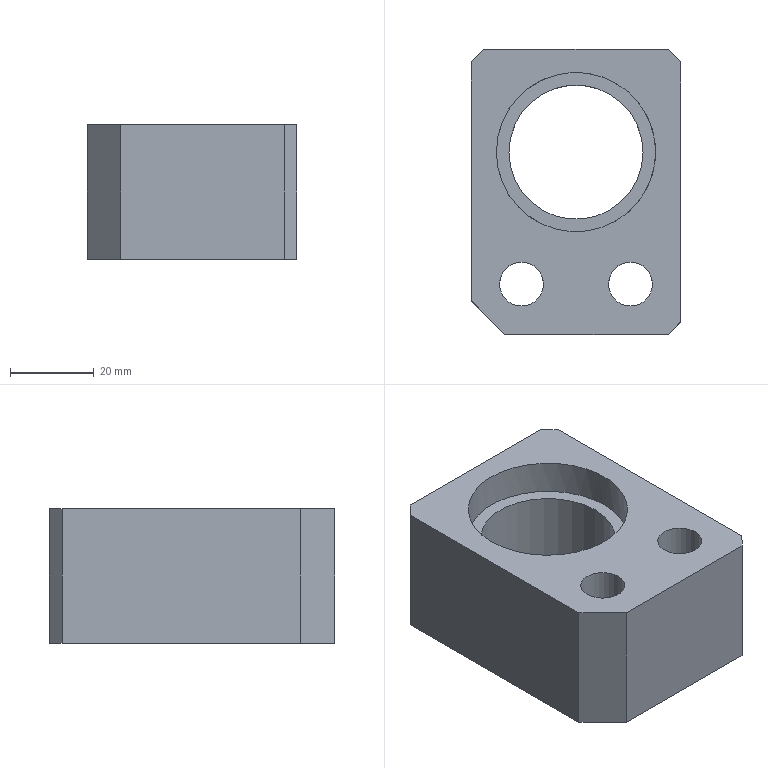Part | STEP file | lll_id3542_x_t | 1 solid | 19 faces | box 50 x 68 x 32 mm | volume 68588 mm3 | plane 13 | cylinder 6 | commonest cylinder face diameters 10.5 x2 17 x2 32 x1 38 x1
STEP:
#1=CARTESIAN_POINT('',(3217.117,-235.788,77.5));
#2=VERTEX_POINT('',#1);
#3=CARTESIAN_POINT('',(3222.367,-235.788,77.5));
#4=DIRECTION('',(0.,0.,1.));
#5=DIRECTION('',(-1.,0.,0.));
#6=AXIS2_PLACEMENT_3D('',#3,#4,#5);
#7=CIRCLE('',#6,5.25);
#8=EDGE_CURVE('',#2,#2,#7,.T.);
#9=ORIENTED_EDGE('',*,*,#8,.T.);
#10=EDGE_LOOP('',(#9));
#11=FACE_BOUND('',#10,.T.);
#12=CARTESIAN_POINT('',(3213.867,-235.788,77.5));
#13=VERTEX_POINT('',#12);
#14=CARTESIAN_POINT('',(3222.367,-235.788,77.5));
#15=DIRECTION('',(0.,0.,1.));
#16=DIRECTION('',(-1.,0.,0.));
#17=AXIS2_PLACEMENT_3D('',#14,#15,#16);
#18=CIRCLE('',#17,8.5);
#19=EDGE_CURVE('',#13,#13,#18,.T.);
#20=ORIENTED_EDGE('',*,*,#19,.F.);
#21=EDGE_LOOP('',(#20));
#22=FACE_BOUND('',#21,.T.);
#23=CARTESIAN_POINT('',(3222.367,-235.788,77.5));
#24=DIRECTION('',(0.,0.,1.));
#25=DIRECTION('',(1.,0.,0.));
#26=AXIS2_PLACEMENT_3D('',#23,#24,#25);
#27=PLANE('',#26);
#28=ADVANCED_FACE('',(#11,#22),#27,.F.);
#29=CARTESIAN_POINT('',(3254.367,-204.288,84.3));
#30=VERTEX_POINT('',#29);
#31=CARTESIAN_POINT('',(3235.367,-204.288,84.3));
#32=DIRECTION('',(0.,0.,1.));
#33=DIRECTION('',(1.,0.,0.));
#34=AXIS2_PLACEMENT_3D('',#31,#32,#33);
#35=CIRCLE('',#34,19.);
#36=EDGE_CURVE('',#30,#30,#35,.T.);
#37=ORIENTED_EDGE('',*,*,#36,.T.);
#38=EDGE_LOOP('',(#37));
#39=FACE_BOUND('',#38,.T.);
#40=CARTESIAN_POINT('',(3251.367,-204.288,84.3));
#41=VERTEX_POINT('',#40);
#42=CARTESIAN_POINT('',(3235.367,-204.288,84.3));
#43=DIRECTION('',(0.,0.,1.));
#44=DIRECTION('',(1.,0.,0.));
#45=AXIS2_PLACEMENT_3D('',#42,#43,#44);
#46=CIRCLE('',#45,16.);
#47=EDGE_CURVE('',#41,#41,#46,.T.);
#48=ORIENTED_EDGE('',*,*,#47,.F.);
#49=EDGE_LOOP('',(#48));
#50=FACE_BOUND('',#49,.T.);
#51=CARTESIAN_POINT('',(3235.367,-213.038,84.3));
#52=DIRECTION('',(0.,0.,-1.));
#53=DIRECTION('',(0.,-1.,0.));
#54=AXIS2_PLACEMENT_3D('',#51,#52,#53);
#55=PLANE('',#54);
#56=ADVANCED_FACE('',(#39,#50),#55,.F.);
#57=ORIENTED_EDGE('',*,*,#19,.T.);
#58=EDGE_LOOP('',(#57));
#59=FACE_BOUND('',#58,.T.);
#60=CARTESIAN_POINT('',(3213.867,-235.788,60.5));
#61=VERTEX_POINT('',#60);
#62=CARTESIAN_POINT('',(3222.367,-235.788,60.5));
#63=DIRECTION('',(0.,0.,-1.));
#64=DIRECTION('',(-1.,0.,0.));
#65=AXIS2_PLACEMENT_3D('',#62,#63,#64);
#66=CIRCLE('',#65,8.5);
#67=EDGE_CURVE('',#61,#61,#66,.T.);
#68=ORIENTED_EDGE('',*,*,#67,.T.);
#69=EDGE_LOOP('',(#68));
#70=FACE_BOUND('',#69,.T.);
#71=CARTESIAN_POINT('',(3222.367,-235.788,60.5));
#72=DIRECTION('',(0.,0.,1.));
#73=DIRECTION('',(1.,0.,0.));
#74=AXIS2_PLACEMENT_3D('',#71,#72,#73);
#75=CYLINDRICAL_SURFACE('',#74,8.5);
#76=ADVANCED_FACE('',(#59,#70),#75,.F.);
#77=CARTESIAN_POINT('',(3210.367,-182.788,60.5));
#78=VERTEX_POINT('',#77);
#79=CARTESIAN_POINT('',(3213.367,-179.788,60.5));
#80=VERTEX_POINT('',#79);
#81=CARTESIAN_POINT('',(3229.549,-163.605,60.5));
#82=DIRECTION('',(0.7071,0.7071,0.));
#83=VECTOR('',#82,1.);
#84=LINE('',#81,#83);
#85=EDGE_CURVE('',#78,#80,#84,.T.);
#86=ORIENTED_EDGE('',*,*,#85,.F.);
#87=CARTESIAN_POINT('',(3210.367,-182.788,92.5));
#88=VERTEX_POINT('',#87);
#89=CARTESIAN_POINT('',(3210.367,-182.788,-8.5));
#90=DIRECTION('',(0.,0.,-1.));
#91=VECTOR('',#90,1.);
#92=LINE('',#89,#91);
#93=EDGE_CURVE('',#88,#78,#92,.T.);
#94=ORIENTED_EDGE('',*,*,#93,.F.);
#95=CARTESIAN_POINT('',(3213.367,-179.788,92.5));
#96=VERTEX_POINT('',#95);
#97=CARTESIAN_POINT('',(3229.549,-163.605,92.5));
#98=DIRECTION('',(-0.7071,-0.7071,0.));
#99=VECTOR('',#98,1.);
#100=LINE('',#97,#99);
#101=EDGE_CURVE('',#96,#88,#100,.T.);
#102=ORIENTED_EDGE('',*,*,#101,.F.);
#103=CARTESIAN_POINT('',(3213.367,-179.788,-8.5));
#104=DIRECTION('',(0.,0.,1.));
#105=VECTOR('',#104,1.);
#106=LINE('',#103,#105);
#107=EDGE_CURVE('',#80,#96,#106,.T.);
#108=ORIENTED_EDGE('',*,*,#107,.F.);
#109=EDGE_LOOP('',(#86,#94,#102,#108));
#110=FACE_OUTER_BOUND('',#109,.T.);
#111=CARTESIAN_POINT('',(3213.367,-179.788,-8.5));
#112=DIRECTION('',(0.7071,-0.7071,0.));
#113=DIRECTION('',(0.,0.,1.));
#114=AXIS2_PLACEMENT_3D('',#111,#112,#113);
#115=PLANE('',#114);
#116=ADVANCED_FACE('',(#110),#115,.F.);
#117=CARTESIAN_POINT('',(3257.367,-179.788,60.5));
#118=VERTEX_POINT('',#117);
#119=CARTESIAN_POINT('',(3298.557,-179.788,60.5));
#120=DIRECTION('',(1.,0.,0.));
#121=VECTOR('',#120,1.);
#122=LINE('',#119,#121);
#123=EDGE_CURVE('',#80,#118,#122,.T.);
#124=ORIENTED_EDGE('',*,*,#123,.F.);
#125=ORIENTED_EDGE('',*,*,#107,.T.);
#126=CARTESIAN_POINT('',(3257.367,-179.788,92.5));
#127=VERTEX_POINT('',#126);
#128=CARTESIAN_POINT('',(3235.367,-179.788,92.5));
#129=DIRECTION('',(-1.,0.,0.));
#130=VECTOR('',#129,1.);
#131=LINE('',#128,#130);
#132=EDGE_CURVE('',#127,#96,#131,.T.);
#133=ORIENTED_EDGE('',*,*,#132,.F.);
#134=CARTESIAN_POINT('',(3257.367,-179.788,-8.5));
#135=DIRECTION('',(0.,0.,1.));
#136=VECTOR('',#135,1.);
#137=LINE('',#134,#136);
#138=EDGE_CURVE('',#118,#127,#137,.T.);
#139=ORIENTED_EDGE('',*,*,#138,.F.);
#140=EDGE_LOOP('',(#124,#125,#133,#139));
#141=FACE_OUTER_BOUND('',#140,.T.);
#142=CARTESIAN_POINT('',(3235.367,-179.788,-8.5));
#143=DIRECTION('',(0.,1.,0.));
#144=DIRECTION('',(0.,0.,-1.));
#145=AXIS2_PLACEMENT_3D('',#142,#143,#144);
#146=PLANE('',#145);
#147=ADVANCED_FACE('',(#141),#146,.T.);
#148=CARTESIAN_POINT('',(3260.367,-182.788,92.5));
#149=VERTEX_POINT('',#148);
#150=CARTESIAN_POINT('',(3260.367,-182.788,92.5));
#151=DIRECTION('',(0.7071,-0.7071,0.));
#152=VECTOR('',#151,1.);
#153=LINE('',#150,#152);
#154=EDGE_CURVE('',#127,#149,#153,.T.);
#155=ORIENTED_EDGE('',*,*,#154,.T.);
#156=CARTESIAN_POINT('',(3260.367,-182.788,60.5));
#157=VERTEX_POINT('',#156);
#158=CARTESIAN_POINT('',(3260.367,-182.788,-8.5));
#159=DIRECTION('',(0.,0.,-1.));
#160=VECTOR('',#159,1.);
#161=LINE('',#158,#160);
#162=EDGE_CURVE('',#149,#157,#161,.T.);
#163=ORIENTED_EDGE('',*,*,#162,.T.);
#164=CARTESIAN_POINT('',(3255.417,-177.838,60.5));
#165=DIRECTION('',(-0.7071,0.7071,0.));
#166=VECTOR('',#165,1.);
#167=LINE('',#164,#166);
#168=EDGE_CURVE('',#157,#118,#167,.T.);
#169=ORIENTED_EDGE('',*,*,#168,.T.);
#170=ORIENTED_EDGE('',*,*,#138,.T.);
#171=EDGE_LOOP('',(#155,#163,#169,#170));
#172=FACE_OUTER_BOUND('',#171,.T.);
#173=CARTESIAN_POINT('',(3260.367,-182.788,-8.5));
#174=DIRECTION('',(-0.7071,-0.7071,0.));
#175=DIRECTION('',(0.7071,-0.7071,0.));
#176=AXIS2_PLACEMENT_3D('',#173,#174,#175);
#177=PLANE('',#176);
#178=ADVANCED_FACE('',(#172),#177,.F.);
#179=CARTESIAN_POINT('',(3260.367,-244.788,60.5));
#180=VERTEX_POINT('',#179);
#181=CARTESIAN_POINT('',(3260.367,-230.563,60.5));
#182=DIRECTION('',(0.,-1.,0.));
#183=VECTOR('',#182,1.);
#184=LINE('',#181,#183);
#185=EDGE_CURVE('',#157,#180,#184,.T.);
#186=ORIENTED_EDGE('',*,*,#185,.F.);
#187=ORIENTED_EDGE('',*,*,#162,.F.);
#188=CARTESIAN_POINT('',(3260.367,-244.788,92.5));
#189=VERTEX_POINT('',#188);
#190=CARTESIAN_POINT('',(3260.367,-235.513,92.5));
#191=DIRECTION('',(0.,1.,0.));
#192=VECTOR('',#191,1.);
#193=LINE('',#190,#192);
#194=EDGE_CURVE('',#189,#149,#193,.T.);
#195=ORIENTED_EDGE('',*,*,#194,.F.);
#196=CARTESIAN_POINT('',(3260.367,-244.788,-8.5));
#197=DIRECTION('',(0.,0.,1.));
#198=VECTOR('',#197,1.);
#199=LINE('',#196,#198);
#200=EDGE_CURVE('',#180,#189,#199,.T.);
#201=ORIENTED_EDGE('',*,*,#200,.F.);
#202=EDGE_LOOP('',(#186,#187,#195,#201));
#203=FACE_OUTER_BOUND('',#202,.T.);
#204=CARTESIAN_POINT('',(3260.367,-204.288,-8.5));
#205=DIRECTION('',(1.,0.,0.));
#206=DIRECTION('',(0.,0.,-1.));
#207=AXIS2_PLACEMENT_3D('',#204,#205,#206);
#208=PLANE('',#207);
#209=ADVANCED_FACE('',(#203),#208,.T.);
#210=CARTESIAN_POINT('',(3257.367,-247.788,92.5));
#211=VERTEX_POINT('',#210);
#212=CARTESIAN_POINT('',(3257.367,-247.788,92.5));
#213=DIRECTION('',(-0.7071,-0.7071,0.));
#214=VECTOR('',#213,1.);
#215=LINE('',#212,#214);
#216=EDGE_CURVE('',#189,#211,#215,.T.);
#217=ORIENTED_EDGE('',*,*,#216,.T.);
#218=CARTESIAN_POINT('',(3257.367,-247.788,60.5));
#219=VERTEX_POINT('',#218);
#220=CARTESIAN_POINT('',(3257.367,-247.788,-8.5));
#221=DIRECTION('',(0.,0.,-1.));
#222=VECTOR('',#221,1.);
#223=LINE('',#220,#222);
#224=EDGE_CURVE('',#211,#219,#223,.T.);
#225=ORIENTED_EDGE('',*,*,#224,.T.);
#226=CARTESIAN_POINT('',(3257.367,-247.788,60.5));
#227=DIRECTION('',(0.7071,0.7071,0.));
#228=VECTOR('',#227,1.);
#229=LINE('',#226,#228);
#230=EDGE_CURVE('',#219,#180,#229,.T.);
#231=ORIENTED_EDGE('',*,*,#230,.T.);
#232=ORIENTED_EDGE('',*,*,#200,.T.);
#233=EDGE_LOOP('',(#217,#225,#231,#232));
#234=FACE_OUTER_BOUND('',#233,.T.);
#235=CARTESIAN_POINT('',(3257.367,-247.788,-8.5));
#236=DIRECTION('',(-0.7071,0.7071,0.));
#237=DIRECTION('',(-0.7071,-0.7071,0.));
#238=AXIS2_PLACEMENT_3D('',#235,#236,#237);
#239=PLANE('',#238);
#240=ADVANCED_FACE('',(#234),#239,.F.);
#241=CARTESIAN_POINT('',(3218.367,-247.788,92.5));
#242=VERTEX_POINT('',#241);
#243=CARTESIAN_POINT('',(3235.367,-247.788,92.5));
#244=DIRECTION('',(1.,0.,0.));
#245=VECTOR('',#244,1.);
#246=LINE('',#243,#245);
#247=EDGE_CURVE('',#242,#211,#246,.T.);
#248=ORIENTED_EDGE('',*,*,#247,.F.);
#249=CARTESIAN_POINT('',(3218.367,-247.788,60.5));
#250=VERTEX_POINT('',#249);
#251=CARTESIAN_POINT('',(3218.367,-247.788,-8.5));
#252=DIRECTION('',(0.,0.,-1.));
#253=VECTOR('',#252,1.);
#254=LINE('',#251,#253);
#255=EDGE_CURVE('',#242,#250,#254,.T.);
#256=ORIENTED_EDGE('',*,*,#255,.T.);
#257=CARTESIAN_POINT('',(3298.557,-247.788,60.5));
#258=DIRECTION('',(-1.,0.,0.));
#259=VECTOR('',#258,1.);
#260=LINE('',#257,#259);
#261=EDGE_CURVE('',#219,#250,#260,.T.);
#262=ORIENTED_EDGE('',*,*,#261,.F.);
#263=ORIENTED_EDGE('',*,*,#224,.F.);
#264=EDGE_LOOP('',(#248,#256,#262,#263));
#265=FACE_OUTER_BOUND('',#264,.T.);
#266=CARTESIAN_POINT('',(3235.367,-247.788,-8.5));
#267=DIRECTION('',(0.,-1.,0.));
#268=DIRECTION('',(0.,0.,1.));
#269=AXIS2_PLACEMENT_3D('',#266,#267,#268);
#270=PLANE('',#269);
#271=ADVANCED_FACE('',(#265),#270,.T.);
#272=CARTESIAN_POINT('',(3210.367,-239.788,92.5));
#273=VERTEX_POINT('',#272);
#274=CARTESIAN_POINT('',(3253.774,-283.195,92.5));
#275=DIRECTION('',(0.7071,-0.7071,0.));
#276=VECTOR('',#275,1.);
#277=LINE('',#274,#276);
#278=EDGE_CURVE('',#273,#242,#277,.T.);
#279=ORIENTED_EDGE('',*,*,#278,.F.);
#280=CARTESIAN_POINT('',(3210.367,-239.788,60.5));
#281=VERTEX_POINT('',#280);
#282=CARTESIAN_POINT('',(3210.367,-239.788,-8.5));
#283=DIRECTION('',(0.,0.,1.));
#284=VECTOR('',#283,1.);
#285=LINE('',#282,#284);
#286=EDGE_CURVE('',#281,#273,#285,.T.);
#287=ORIENTED_EDGE('',*,*,#286,.F.);
#288=CARTESIAN_POINT('',(3248.825,-278.245,60.5));
#289=DIRECTION('',(-0.7071,0.7071,0.));
#290=VECTOR('',#289,1.);
#291=LINE('',#288,#290);
#292=EDGE_CURVE('',#250,#281,#291,.T.);
#293=ORIENTED_EDGE('',*,*,#292,.F.);
#294=ORIENTED_EDGE('',*,*,#255,.F.);
#295=EDGE_LOOP('',(#279,#287,#293,#294));
#296=FACE_OUTER_BOUND('',#295,.T.);
#297=CARTESIAN_POINT('',(3218.367,-247.788,-8.5));
#298=DIRECTION('',(0.7071,0.7071,0.));
#299=DIRECTION('',(0.,0.,-1.));
#300=AXIS2_PLACEMENT_3D('',#297,#298,#299);
#301=PLANE('',#300);
#302=ADVANCED_FACE('',(#296),#301,.F.);
#303=CARTESIAN_POINT('',(3210.367,-230.563,60.5));
#304=DIRECTION('',(0.,1.,0.));
#305=VECTOR('',#304,1.);
#306=LINE('',#303,#305);
#307=EDGE_CURVE('',#281,#78,#306,.T.);
#308=ORIENTED_EDGE('',*,*,#307,.F.);
#309=ORIENTED_EDGE('',*,*,#286,.T.);
#310=CARTESIAN_POINT('',(3210.367,-230.563,92.5));
#311=DIRECTION('',(0.,-1.,0.));
#312=VECTOR('',#311,1.);
#313=LINE('',#310,#312);
#314=EDGE_CURVE('',#88,#273,#313,.T.);
#315=ORIENTED_EDGE('',*,*,#314,.F.);
#316=ORIENTED_EDGE('',*,*,#93,.T.);
#317=EDGE_LOOP('',(#308,#309,#315,#316));
#318=FACE_OUTER_BOUND('',#317,.T.);
#319=CARTESIAN_POINT('',(3210.367,-199.338,-8.5));
#320=DIRECTION('',(-1.,0.,0.));
#321=DIRECTION('',(0.,0.,1.));
#322=AXIS2_PLACEMENT_3D('',#319,#320,#321);
#323=PLANE('',#322);
#324=ADVANCED_FACE('',(#318),#323,.T.);
#325=CARTESIAN_POINT('',(3217.117,-235.788,92.5));
#326=VERTEX_POINT('',#325);
#327=CARTESIAN_POINT('',(3222.367,-235.788,92.5));
#328=DIRECTION('',(0.,0.,-1.));
#329=DIRECTION('',(-1.,0.,0.));
#330=AXIS2_PLACEMENT_3D('',#327,#328,#329);
#331=CIRCLE('',#330,5.25);
#332=EDGE_CURVE('',#326,#326,#331,.T.);
#333=ORIENTED_EDGE('',*,*,#332,.F.);
#334=EDGE_LOOP('',(#333));
#335=FACE_BOUND('',#334,.T.);
#336=ORIENTED_EDGE('',*,*,#8,.F.);
#337=EDGE_LOOP('',(#336));
#338=FACE_BOUND('',#337,.T.);
#339=CARTESIAN_POINT('',(3222.367,-235.788,160.5));
#340=DIRECTION('',(0.,0.,1.));
#341=DIRECTION('',(1.,0.,0.));
#342=AXIS2_PLACEMENT_3D('',#339,#340,#341);
#343=CYLINDRICAL_SURFACE('',#342,5.25);
#344=ADVANCED_FACE('',(#335,#338),#343,.F.);
#345=CARTESIAN_POINT('',(3216.367,-204.288,92.5));
#346=VERTEX_POINT('',#345);
#347=CARTESIAN_POINT('',(3235.367,-204.288,92.5));
#348=DIRECTION('',(0.,0.,-1.));
#349=DIRECTION('',(-1.,0.,0.));
#350=AXIS2_PLACEMENT_3D('',#347,#348,#349);
#351=CIRCLE('',#350,19.);
#352=EDGE_CURVE('',#346,#346,#351,.T.);
#353=ORIENTED_EDGE('',*,*,#352,.F.);
#354=EDGE_LOOP('',(#353));
#355=FACE_BOUND('',#354,.T.);
#356=ORIENTED_EDGE('',*,*,#36,.F.);
#357=EDGE_LOOP('',(#356));
#358=FACE_BOUND('',#357,.T.);
#359=CARTESIAN_POINT('',(3235.367,-204.288,90.));
#360=DIRECTION('',(0.,0.,-1.));
#361=DIRECTION('',(0.,1.,0.));
#362=AXIS2_PLACEMENT_3D('',#359,#360,#361);
#363=CYLINDRICAL_SURFACE('',#362,19.);
#364=ADVANCED_FACE('',(#355,#358),#363,.F.);
#365=CARTESIAN_POINT('',(3253.617,-235.788,92.5));
#366=VERTEX_POINT('',#365);
#367=CARTESIAN_POINT('',(3248.367,-235.788,92.5));
#368=DIRECTION('',(0.,0.,1.));
#369=DIRECTION('',(1.,0.,0.));
#370=AXIS2_PLACEMENT_3D('',#367,#368,#369);
#371=CIRCLE('',#370,5.25);
#372=EDGE_CURVE('',#366,#366,#371,.T.);
#373=ORIENTED_EDGE('',*,*,#372,.F.);
#374=EDGE_LOOP('',(#373));
#375=FACE_BOUND('',#374,.T.);
#376=ORIENTED_EDGE('',*,*,#352,.T.);
#377=EDGE_LOOP('',(#376));
#378=FACE_BOUND('',#377,.T.);
#379=ORIENTED_EDGE('',*,*,#332,.T.);
#380=EDGE_LOOP('',(#379));
#381=FACE_BOUND('',#380,.T.);
#382=ORIENTED_EDGE('',*,*,#314,.T.);
#383=ORIENTED_EDGE('',*,*,#278,.T.);
#384=ORIENTED_EDGE('',*,*,#247,.T.);
#385=ORIENTED_EDGE('',*,*,#216,.F.);
#386=ORIENTED_EDGE('',*,*,#194,.T.);
#387=ORIENTED_EDGE('',*,*,#154,.F.);
#388=ORIENTED_EDGE('',*,*,#132,.T.);
#389=ORIENTED_EDGE('',*,*,#101,.T.);
#390=EDGE_LOOP('',(#382,#383,#384,#385,#386,#387,#388,#389));
#391=FACE_BOUND('',#390,.T.);
#392=CARTESIAN_POINT('',(3303.507,-235.513,92.5));
#393=DIRECTION('',(0.,0.,1.));
#394=DIRECTION('',(1.,0.,0.));
#395=AXIS2_PLACEMENT_3D('',#392,#393,#394);
#396=PLANE('',#395);
#397=ADVANCED_FACE('',(#375,#378,#381,#391),#396,.T.);
#398=CARTESIAN_POINT('',(3219.367,-204.288,60.5));
#399=VERTEX_POINT('',#398);
#400=CARTESIAN_POINT('',(3235.367,-204.288,60.5));
#401=DIRECTION('',(0.,0.,1.));
#402=DIRECTION('',(-1.,0.,0.));
#403=AXIS2_PLACEMENT_3D('',#400,#401,#402);
#404=CIRCLE('',#403,16.);
#405=EDGE_CURVE('',#399,#399,#404,.T.);
#406=ORIENTED_EDGE('',*,*,#405,.F.);
#407=EDGE_LOOP('',(#406));
#408=FACE_BOUND('',#407,.T.);
#409=ORIENTED_EDGE('',*,*,#47,.T.);
#410=EDGE_LOOP('',(#409));
#411=FACE_BOUND('',#410,.T.);
#412=CARTESIAN_POINT('',(3235.367,-204.288,44.8));
#413=DIRECTION('',(0.,0.,-1.));
#414=DIRECTION('',(0.,1.,0.));
#415=AXIS2_PLACEMENT_3D('',#412,#413,#414);
#416=CYLINDRICAL_SURFACE('',#415,16.);
#417=ADVANCED_FACE('',(#408,#411),#416,.F.);
#418=CARTESIAN_POINT('',(3256.867,-235.788,60.5));
#419=VERTEX_POINT('',#418);
#420=CARTESIAN_POINT('',(3248.367,-235.788,60.5));
#421=DIRECTION('',(0.,0.,-1.));
#422=DIRECTION('',(1.,0.,0.));
#423=AXIS2_PLACEMENT_3D('',#420,#421,#422);
#424=CIRCLE('',#423,8.5);
#425=EDGE_CURVE('',#419,#419,#424,.T.);
#426=ORIENTED_EDGE('',*,*,#425,.F.);
#427=EDGE_LOOP('',(#426));
#428=FACE_BOUND('',#427,.T.);
#429=ORIENTED_EDGE('',*,*,#405,.T.);
#430=EDGE_LOOP('',(#429));
#431=FACE_BOUND('',#430,.T.);
#432=ORIENTED_EDGE('',*,*,#261,.T.);
#433=ORIENTED_EDGE('',*,*,#292,.T.);
#434=ORIENTED_EDGE('',*,*,#307,.T.);
#435=ORIENTED_EDGE('',*,*,#85,.T.);
#436=ORIENTED_EDGE('',*,*,#123,.T.);
#437=ORIENTED_EDGE('',*,*,#168,.F.);
#438=ORIENTED_EDGE('',*,*,#185,.T.);
#439=ORIENTED_EDGE('',*,*,#230,.F.);
#440=EDGE_LOOP('',(#432,#433,#434,#435,#436,#437,#438,#439));
#441=FACE_BOUND('',#440,.T.);
#442=ORIENTED_EDGE('',*,*,#67,.F.);
#443=EDGE_LOOP('',(#442));
#444=FACE_BOUND('',#443,.T.);
#445=CARTESIAN_POINT('',(3298.557,-230.563,60.5));
#446=DIRECTION('',(0.,0.,1.));
#447=DIRECTION('',(1.,0.,0.));
#448=AXIS2_PLACEMENT_3D('',#445,#446,#447);
#449=PLANE('',#448);
#450=ADVANCED_FACE('',(#428,#431,#441,#444),#449,.F.);
#451=CARTESIAN_POINT('',(3253.617,-235.788,77.5));
#452=VERTEX_POINT('',#451);
#453=CARTESIAN_POINT('',(3248.367,-235.788,77.5));
#454=DIRECTION('',(0.,0.,1.));
#455=DIRECTION('',(1.,0.,0.));
#456=AXIS2_PLACEMENT_3D('',#453,#454,#455);
#457=CIRCLE('',#456,5.25);
#458=EDGE_CURVE('',#452,#452,#457,.T.);
#459=ORIENTED_EDGE('',*,*,#458,.T.);
#460=EDGE_LOOP('',(#459));
#461=FACE_BOUND('',#460,.T.);
#462=CARTESIAN_POINT('',(3256.867,-235.788,77.5));
#463=VERTEX_POINT('',#462);
#464=CARTESIAN_POINT('',(3248.367,-235.788,77.5));
#465=DIRECTION('',(0.,0.,1.));
#466=DIRECTION('',(1.,0.,0.));
#467=AXIS2_PLACEMENT_3D('',#464,#465,#466);
#468=CIRCLE('',#467,8.5);
#469=EDGE_CURVE('',#463,#463,#468,.T.);
#470=ORIENTED_EDGE('',*,*,#469,.F.);
#471=EDGE_LOOP('',(#470));
#472=FACE_BOUND('',#471,.T.);
#473=CARTESIAN_POINT('',(3248.367,-235.788,77.5));
#474=DIRECTION('',(0.,0.,1.));
#475=DIRECTION('',(-1.,0.,0.));
#476=AXIS2_PLACEMENT_3D('',#473,#474,#475);
#477=PLANE('',#476);
#478=ADVANCED_FACE('',(#461,#472),#477,.F.);
#479=ORIENTED_EDGE('',*,*,#372,.T.);
#480=EDGE_LOOP('',(#479));
#481=FACE_BOUND('',#480,.T.);
#482=ORIENTED_EDGE('',*,*,#458,.F.);
#483=EDGE_LOOP('',(#482));
#484=FACE_BOUND('',#483,.T.);
#485=CARTESIAN_POINT('',(3248.367,-235.788,160.5));
#486=DIRECTION('',(0.,0.,1.));
#487=DIRECTION('',(-1.,0.,0.));
#488=AXIS2_PLACEMENT_3D('',#485,#486,#487);
#489=CYLINDRICAL_SURFACE('',#488,5.25);
#490=ADVANCED_FACE('',(#481,#484),#489,.F.);
#491=ORIENTED_EDGE('',*,*,#469,.T.);
#492=EDGE_LOOP('',(#491));
#493=FACE_BOUND('',#492,.T.);
#494=ORIENTED_EDGE('',*,*,#425,.T.);
#495=EDGE_LOOP('',(#494));
#496=FACE_BOUND('',#495,.T.);
#497=CARTESIAN_POINT('',(3248.367,-235.788,60.5));
#498=DIRECTION('',(0.,0.,1.));
#499=DIRECTION('',(-1.,0.,0.));
#500=AXIS2_PLACEMENT_3D('',#497,#498,#499);
#501=CYLINDRICAL_SURFACE('',#500,8.5);
#502=ADVANCED_FACE('',(#493,#496),#501,.F.);
#503=CLOSED_SHELL('',(#28,#56,#76,#116,#147,#178,#209,#240,#271,#302,#324,#344,#364,#397,#417,#450,#478,#490,#502));
#504=MANIFOLD_SOLID_BREP('',#503);
#505=(LENGTH_UNIT()NAMED_UNIT(*)SI_UNIT(.MILLI.,.METRE.));
#506=UNCERTAINTY_MEASURE_WITH_UNIT(LENGTH_MEASURE(0.00002),#505,'','');
#507=(NAMED_UNIT(*)PLANE_ANGLE_UNIT()SI_UNIT($,.RADIAN.));
#508=PLANE_ANGLE_MEASURE_WITH_UNIT(PLANE_ANGLE_MEASURE(0.01745),#507);
#509=DIMENSIONAL_EXPONENTS(0.,0.,0.,0.,0.,0.,0.);
#510=(CONVERSION_BASED_UNIT('DEGREE',#508)NAMED_UNIT(#509)PLANE_ANGLE_UNIT());
#511=(NAMED_UNIT(*)SI_UNIT($,.STERADIAN.)SOLID_ANGLE_UNIT());
#512=(GEOMETRIC_REPRESENTATION_CONTEXT(3)GLOBAL_UNCERTAINTY_ASSIGNED_CONTEXT((#506))GLOBAL_UNIT_ASSIGNED_CONTEXT((#505,#510,#511))REPRESENTATION_CONTEXT('',''));
#513=ADVANCED_BREP_SHAPE_REPRESENTATION('',(#504),#512);